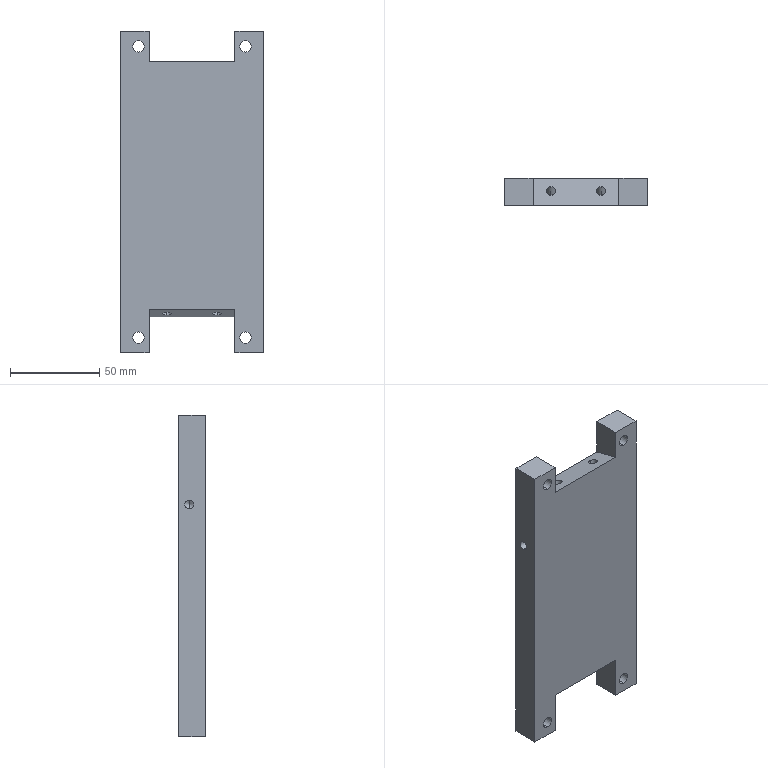Part | SolidWorks | features BaseBody 1 | 1 solid | 46 faces | box 80 x 15 x 180 mm | volume 182488 mm3 | cylinder 20 | plane 14 | cone 12 | commonest cylinder face diameters 5 x12 6.4 x8
STEP:
#1=CARTESIAN_POINT('',(14.,12.806,-50.107));
#2=VERTEX_POINT('',#1);
#3=CARTESIAN_POINT('',(14.,10.002,-50.911));
#4=VERTEX_POINT('',#3);
#5=CARTESIAN_POINT('',(14.,10.002,-50.911));
#6=DIRECTION('',(0.,-0.9613,-0.2756));
#7=VECTOR('',#6,1000.);
#8=LINE('',#5,#7);
#9=EDGE_CURVE('',#2,#4,#8,.T.);
#10=ORIENTED_EDGE('',*,*,#9,.F.);
#11=CARTESIAN_POINT('',(14.,14.832,-52.205));
#12=VERTEX_POINT('',#11);
#13=CARTESIAN_POINT('',(14.,14.832,-52.205));
#14=DIRECTION('',(0.,0.6947,-0.7193));
#15=VECTOR('',#14,1000.);
#16=LINE('',#13,#15);
#17=EDGE_CURVE('',#2,#12,#16,.T.);
#18=ORIENTED_EDGE('',*,*,#17,.T.);
#19=CARTESIAN_POINT('',(14.,12.417,-51.558));
#20=DIRECTION('',(0.,-0.2588,-0.9659));
#21=DIRECTION('',(0.,0.9659,-0.2588));
#22=AXIS2_PLACEMENT_3D('',#19,#20,#21);
#23=CIRCLE('',#22,2.5);
#24=EDGE_CURVE('',#12,#4,#23,.T.);
#25=ORIENTED_EDGE('',*,*,#24,.T.);
#26=EDGE_LOOP('',(#10,#18,#25));
#27=FACE_OUTER_BOUND('',#26,.T.);
#28=CARTESIAN_POINT('',(14.,12.417,-51.558));
#29=DIRECTION('',(0.,-0.2588,-0.9659));
#30=DIRECTION('',(0.,0.9659,-0.2588));
#31=AXIS2_PLACEMENT_3D('',#28,#29,#30);
#32=CONICAL_SURFACE('',#31,2.5,1.03);
#33=ADVANCED_FACE('',(#27),#32,.F.);
#34=CARTESIAN_POINT('',(-14.,12.806,-50.107));
#35=VERTEX_POINT('',#34);
#36=CARTESIAN_POINT('',(-14.,10.002,-50.911));
#37=VERTEX_POINT('',#36);
#38=CARTESIAN_POINT('',(-14.,10.002,-50.911));
#39=DIRECTION('',(0.,-0.9613,-0.2756));
#40=VECTOR('',#39,1000.);
#41=LINE('',#38,#40);
#42=EDGE_CURVE('',#35,#37,#41,.T.);
#43=ORIENTED_EDGE('',*,*,#42,.F.);
#44=CARTESIAN_POINT('',(-14.,14.832,-52.205));
#45=VERTEX_POINT('',#44);
#46=CARTESIAN_POINT('',(-14.,14.832,-52.205));
#47=DIRECTION('',(0.,0.6947,-0.7193));
#48=VECTOR('',#47,1000.);
#49=LINE('',#46,#48);
#50=EDGE_CURVE('',#35,#45,#49,.T.);
#51=ORIENTED_EDGE('',*,*,#50,.T.);
#52=CARTESIAN_POINT('',(-14.,12.417,-51.558));
#53=DIRECTION('',(0.,-0.2588,-0.9659));
#54=DIRECTION('',(0.,0.9659,-0.2588));
#55=AXIS2_PLACEMENT_3D('',#52,#53,#54);
#56=CIRCLE('',#55,2.5);
#57=EDGE_CURVE('',#45,#37,#56,.T.);
#58=ORIENTED_EDGE('',*,*,#57,.T.);
#59=EDGE_LOOP('',(#43,#51,#58));
#60=FACE_OUTER_BOUND('',#59,.T.);
#61=CARTESIAN_POINT('',(-14.,12.417,-51.558));
#62=DIRECTION('',(0.,-0.2588,-0.9659));
#63=DIRECTION('',(0.,0.9659,-0.2588));
#64=AXIS2_PLACEMENT_3D('',#61,#62,#63);
#65=CONICAL_SURFACE('',#64,2.5,1.03);
#66=ADVANCED_FACE('',(#60),#65,.F.);
#67=CARTESIAN_POINT('',(-21.498,9.,40.));
#68=VERTEX_POINT('',#67);
#69=CARTESIAN_POINT('',(-23.,9.,37.5));
#70=VERTEX_POINT('',#69);
#71=CARTESIAN_POINT('',(-23.,9.,37.5));
#72=DIRECTION('',(-0.515,0.,-0.8572));
#73=VECTOR('',#72,1000.);
#74=LINE('',#71,#73);
#75=EDGE_CURVE('',#68,#70,#74,.T.);
#76=ORIENTED_EDGE('',*,*,#75,.F.);
#77=CARTESIAN_POINT('',(-23.,9.,42.5));
#78=VERTEX_POINT('',#77);
#79=CARTESIAN_POINT('',(-23.,9.,42.5));
#80=DIRECTION('',(-0.515,0.,0.8572));
#81=VECTOR('',#80,1000.);
#82=LINE('',#79,#81);
#83=EDGE_CURVE('',#68,#78,#82,.T.);
#84=ORIENTED_EDGE('',*,*,#83,.T.);
#85=CARTESIAN_POINT('',(-23.,9.,40.));
#86=DIRECTION('',(-1.,0.,0.));
#87=DIRECTION('',(0.,0.,1.));
#88=AXIS2_PLACEMENT_3D('',#85,#86,#87);
#89=CIRCLE('',#88,2.5);
#90=EDGE_CURVE('',#78,#70,#89,.T.);
#91=ORIENTED_EDGE('',*,*,#90,.T.);
#92=EDGE_LOOP('',(#76,#84,#91));
#93=FACE_OUTER_BOUND('',#92,.T.);
#94=CARTESIAN_POINT('',(-23.,9.,40.));
#95=DIRECTION('',(-1.,0.,0.));
#96=DIRECTION('',(0.,0.,1.));
#97=AXIS2_PLACEMENT_3D('',#94,#95,#96);
#98=CONICAL_SURFACE('',#97,2.5,1.03);
#99=ADVANCED_FACE('',(#93),#98,.F.);
#100=CARTESIAN_POINT('',(14.,3.228,53.149));
#101=VERTEX_POINT('',#100);
#102=CARTESIAN_POINT('',(14.,6.032,53.953));
#103=VERTEX_POINT('',#102);
#104=CARTESIAN_POINT('',(14.,6.032,53.953));
#105=DIRECTION('',(0.,0.9613,0.2756));
#106=VECTOR('',#105,1000.);
#107=LINE('',#104,#106);
#108=EDGE_CURVE('',#101,#103,#107,.T.);
#109=ORIENTED_EDGE('',*,*,#108,.F.);
#110=CARTESIAN_POINT('',(14.,1.202,55.247));
#111=VERTEX_POINT('',#110);
#112=CARTESIAN_POINT('',(14.,1.202,55.247));
#113=DIRECTION('',(0.,-0.6947,0.7193));
#114=VECTOR('',#113,1000.);
#115=LINE('',#112,#114);
#116=EDGE_CURVE('',#101,#111,#115,.T.);
#117=ORIENTED_EDGE('',*,*,#116,.T.);
#118=CARTESIAN_POINT('',(14.,3.617,54.6));
#119=DIRECTION('',(0.,0.2588,0.9659));
#120=DIRECTION('',(0.,-0.9659,0.2588));
#121=AXIS2_PLACEMENT_3D('',#118,#119,#120);
#122=CIRCLE('',#121,2.5);
#123=EDGE_CURVE('',#111,#103,#122,.T.);
#124=ORIENTED_EDGE('',*,*,#123,.T.);
#125=EDGE_LOOP('',(#109,#117,#124));
#126=FACE_OUTER_BOUND('',#125,.T.);
#127=CARTESIAN_POINT('',(14.,3.617,54.6));
#128=DIRECTION('',(0.,0.2588,0.9659));
#129=DIRECTION('',(0.,-0.9659,0.2588));
#130=AXIS2_PLACEMENT_3D('',#127,#128,#129);
#131=CONICAL_SURFACE('',#130,2.5,1.03);
#132=ADVANCED_FACE('',(#126),#131,.F.);
#133=CARTESIAN_POINT('',(-14.,3.228,53.149));
#134=VERTEX_POINT('',#133);
#135=CARTESIAN_POINT('',(-14.,6.032,53.953));
#136=VERTEX_POINT('',#135);
#137=CARTESIAN_POINT('',(-14.,6.032,53.953));
#138=DIRECTION('',(0.,0.9613,0.2756));
#139=VECTOR('',#138,1000.);
#140=LINE('',#137,#139);
#141=EDGE_CURVE('',#134,#136,#140,.T.);
#142=ORIENTED_EDGE('',*,*,#141,.F.);
#143=CARTESIAN_POINT('',(-14.,1.202,55.247));
#144=VERTEX_POINT('',#143);
#145=CARTESIAN_POINT('',(-14.,1.202,55.247));
#146=DIRECTION('',(0.,-0.6947,0.7193));
#147=VECTOR('',#146,1000.);
#148=LINE('',#145,#147);
#149=EDGE_CURVE('',#134,#144,#148,.T.);
#150=ORIENTED_EDGE('',*,*,#149,.T.);
#151=CARTESIAN_POINT('',(-14.,3.617,54.6));
#152=DIRECTION('',(0.,0.2588,0.9659));
#153=DIRECTION('',(0.,-0.9659,0.2588));
#154=AXIS2_PLACEMENT_3D('',#151,#152,#153);
#155=CIRCLE('',#154,2.5);
#156=EDGE_CURVE('',#144,#136,#155,.T.);
#157=ORIENTED_EDGE('',*,*,#156,.T.);
#158=EDGE_LOOP('',(#142,#150,#157));
#159=FACE_OUTER_BOUND('',#158,.T.);
#160=CARTESIAN_POINT('',(-14.,3.617,54.6));
#161=DIRECTION('',(0.,0.2588,0.9659));
#162=DIRECTION('',(0.,-0.9659,0.2588));
#163=AXIS2_PLACEMENT_3D('',#160,#161,#162);
#164=CONICAL_SURFACE('',#163,2.5,1.03);
#165=ADVANCED_FACE('',(#159),#164,.F.);
#166=CARTESIAN_POINT('',(21.498,9.,-60.));
#167=VERTEX_POINT('',#166);
#168=CARTESIAN_POINT('',(23.,9.,-57.5));
#169=VERTEX_POINT('',#168);
#170=CARTESIAN_POINT('',(23.,9.,-57.5));
#171=DIRECTION('',(0.515,0.,0.8572));
#172=VECTOR('',#171,1000.);
#173=LINE('',#170,#172);
#174=EDGE_CURVE('',#167,#169,#173,.T.);
#175=ORIENTED_EDGE('',*,*,#174,.F.);
#176=CARTESIAN_POINT('',(23.,9.,-62.5));
#177=VERTEX_POINT('',#176);
#178=CARTESIAN_POINT('',(23.,9.,-62.5));
#179=DIRECTION('',(0.515,0.,-0.8572));
#180=VECTOR('',#179,1000.);
#181=LINE('',#178,#180);
#182=EDGE_CURVE('',#167,#177,#181,.T.);
#183=ORIENTED_EDGE('',*,*,#182,.T.);
#184=CARTESIAN_POINT('',(23.,9.,-60.));
#185=DIRECTION('',(1.,0.,0.));
#186=DIRECTION('',(0.,0.,-1.));
#187=AXIS2_PLACEMENT_3D('',#184,#185,#186);
#188=CIRCLE('',#187,2.5);
#189=EDGE_CURVE('',#177,#169,#188,.T.);
#190=ORIENTED_EDGE('',*,*,#189,.T.);
#191=EDGE_LOOP('',(#175,#183,#190));
#192=FACE_OUTER_BOUND('',#191,.T.);
#193=CARTESIAN_POINT('',(23.,9.,-60.));
#194=DIRECTION('',(1.,0.,0.));
#195=DIRECTION('',(0.,0.,-1.));
#196=AXIS2_PLACEMENT_3D('',#193,#194,#195);
#197=CONICAL_SURFACE('',#196,2.5,1.03);
#198=ADVANCED_FACE('',(#192),#197,.F.);
#199=CARTESIAN_POINT('',(14.,5.602,-67.332));
#200=VERTEX_POINT('',#199);
#201=CARTESIAN_POINT('',(14.,5.602,-67.332));
#202=DIRECTION('',(0.,-0.2588,-0.9659));
#203=VECTOR('',#202,1000.);
#204=LINE('',#201,#203);
#205=EDGE_CURVE('',#4,#200,#204,.T.);
#206=ORIENTED_EDGE('',*,*,#205,.F.);
#207=ORIENTED_EDGE('',*,*,#24,.F.);
#208=CARTESIAN_POINT('',(14.,10.432,-68.626));
#209=VERTEX_POINT('',#208);
#210=CARTESIAN_POINT('',(14.,10.432,-68.626));
#211=DIRECTION('',(0.,-0.2588,-0.9659));
#212=VECTOR('',#211,1000.);
#213=LINE('',#210,#212);
#214=EDGE_CURVE('',#12,#209,#213,.T.);
#215=ORIENTED_EDGE('',*,*,#214,.T.);
#216=CARTESIAN_POINT('',(14.,8.017,-67.979));
#217=DIRECTION('',(0.,0.2588,0.9659));
#218=DIRECTION('',(0.,0.9659,-0.2588));
#219=AXIS2_PLACEMENT_3D('',#216,#217,#218);
#220=CIRCLE('',#219,2.5);
#221=EDGE_CURVE('',#200,#209,#220,.T.);
#222=ORIENTED_EDGE('',*,*,#221,.F.);
#223=EDGE_LOOP('',(#206,#207,#215,#222));
#224=FACE_OUTER_BOUND('',#223,.T.);
#225=CARTESIAN_POINT('',(14.,8.017,-67.979));
#226=DIRECTION('',(0.,-0.2588,-0.9659));
#227=DIRECTION('',(0.,0.9659,-0.2588));
#228=AXIS2_PLACEMENT_3D('',#225,#226,#227);
#229=CYLINDRICAL_SURFACE('',#228,2.5);
#230=ADVANCED_FACE('',(#224),#229,.F.);
#231=CARTESIAN_POINT('',(-14.,5.602,-67.332));
#232=VERTEX_POINT('',#231);
#233=CARTESIAN_POINT('',(-14.,5.602,-67.332));
#234=DIRECTION('',(0.,-0.2588,-0.9659));
#235=VECTOR('',#234,1000.);
#236=LINE('',#233,#235);
#237=EDGE_CURVE('',#37,#232,#236,.T.);
#238=ORIENTED_EDGE('',*,*,#237,.F.);
#239=ORIENTED_EDGE('',*,*,#57,.F.);
#240=CARTESIAN_POINT('',(-14.,10.432,-68.626));
#241=VERTEX_POINT('',#240);
#242=CARTESIAN_POINT('',(-14.,10.432,-68.626));
#243=DIRECTION('',(0.,-0.2588,-0.9659));
#244=VECTOR('',#243,1000.);
#245=LINE('',#242,#244);
#246=EDGE_CURVE('',#45,#241,#245,.T.);
#247=ORIENTED_EDGE('',*,*,#246,.T.);
#248=CARTESIAN_POINT('',(-14.,8.017,-67.979));
#249=DIRECTION('',(0.,0.2588,0.9659));
#250=DIRECTION('',(0.,0.9659,-0.2588));
#251=AXIS2_PLACEMENT_3D('',#248,#249,#250);
#252=CIRCLE('',#251,2.5);
#253=EDGE_CURVE('',#232,#241,#252,.T.);
#254=ORIENTED_EDGE('',*,*,#253,.F.);
#255=EDGE_LOOP('',(#238,#239,#247,#254));
#256=FACE_OUTER_BOUND('',#255,.T.);
#257=CARTESIAN_POINT('',(-14.,8.017,-67.979));
#258=DIRECTION('',(0.,-0.2588,-0.9659));
#259=DIRECTION('',(0.,0.9659,-0.2588));
#260=AXIS2_PLACEMENT_3D('',#257,#258,#259);
#261=CYLINDRICAL_SURFACE('',#260,2.5);
#262=ADVANCED_FACE('',(#256),#261,.F.);
#263=CARTESIAN_POINT('',(-40.,9.,37.5));
#264=VERTEX_POINT('',#263);
#265=CARTESIAN_POINT('',(-40.,9.,37.5));
#266=DIRECTION('',(-1.,0.,0.));
#267=VECTOR('',#266,1000.);
#268=LINE('',#265,#267);
#269=EDGE_CURVE('',#70,#264,#268,.T.);
#270=ORIENTED_EDGE('',*,*,#269,.F.);
#271=ORIENTED_EDGE('',*,*,#90,.F.);
#272=CARTESIAN_POINT('',(-40.,9.,42.5));
#273=VERTEX_POINT('',#272);
#274=CARTESIAN_POINT('',(-40.,9.,42.5));
#275=DIRECTION('',(-1.,0.,0.));
#276=VECTOR('',#275,1000.);
#277=LINE('',#274,#276);
#278=EDGE_CURVE('',#78,#273,#277,.T.);
#279=ORIENTED_EDGE('',*,*,#278,.T.);
#280=CARTESIAN_POINT('',(-40.,9.,40.));
#281=DIRECTION('',(-1.,0.,0.));
#282=DIRECTION('',(0.,0.,1.));
#283=AXIS2_PLACEMENT_3D('',#280,#281,#282);
#284=CIRCLE('',#283,2.5);
#285=EDGE_CURVE('',#273,#264,#284,.T.);
#286=ORIENTED_EDGE('',*,*,#285,.T.);
#287=EDGE_LOOP('',(#270,#271,#279,#286));
#288=FACE_OUTER_BOUND('',#287,.T.);
#289=CARTESIAN_POINT('',(-40.,9.,40.));
#290=DIRECTION('',(-1.,0.,0.));
#291=DIRECTION('',(0.,0.,1.));
#292=AXIS2_PLACEMENT_3D('',#289,#290,#291);
#293=CYLINDRICAL_SURFACE('',#292,2.5);
#294=ADVANCED_FACE('',(#288),#293,.F.);
#295=CARTESIAN_POINT('',(14.,10.432,70.374));
#296=VERTEX_POINT('',#295);
#297=CARTESIAN_POINT('',(14.,10.432,70.374));
#298=DIRECTION('',(0.,0.2588,0.9659));
#299=VECTOR('',#298,1000.);
#300=LINE('',#297,#299);
#301=EDGE_CURVE('',#103,#296,#300,.T.);
#302=ORIENTED_EDGE('',*,*,#301,.F.);
#303=ORIENTED_EDGE('',*,*,#123,.F.);
#304=CARTESIAN_POINT('',(14.,5.602,71.668));
#305=VERTEX_POINT('',#304);
#306=CARTESIAN_POINT('',(14.,5.602,71.668));
#307=DIRECTION('',(0.,0.2588,0.9659));
#308=VECTOR('',#307,1000.);
#309=LINE('',#306,#308);
#310=EDGE_CURVE('',#111,#305,#309,.T.);
#311=ORIENTED_EDGE('',*,*,#310,.T.);
#312=CARTESIAN_POINT('',(14.,8.017,71.021));
#313=DIRECTION('',(0.,-0.2588,-0.9659));
#314=DIRECTION('',(0.,-0.9659,0.2588));
#315=AXIS2_PLACEMENT_3D('',#312,#313,#314);
#316=CIRCLE('',#315,2.5);
#317=EDGE_CURVE('',#296,#305,#316,.T.);
#318=ORIENTED_EDGE('',*,*,#317,.F.);
#319=EDGE_LOOP('',(#302,#303,#311,#318));
#320=FACE_OUTER_BOUND('',#319,.T.);
#321=CARTESIAN_POINT('',(14.,8.017,71.021));
#322=DIRECTION('',(0.,0.2588,0.9659));
#323=DIRECTION('',(0.,-0.9659,0.2588));
#324=AXIS2_PLACEMENT_3D('',#321,#322,#323);
#325=CYLINDRICAL_SURFACE('',#324,2.5);
#326=ADVANCED_FACE('',(#320),#325,.F.);
#327=CARTESIAN_POINT('',(-14.,10.432,70.374));
#328=VERTEX_POINT('',#327);
#329=CARTESIAN_POINT('',(-14.,10.432,70.374));
#330=DIRECTION('',(0.,0.2588,0.9659));
#331=VECTOR('',#330,1000.);
#332=LINE('',#329,#331);
#333=EDGE_CURVE('',#136,#328,#332,.T.);
#334=ORIENTED_EDGE('',*,*,#333,.F.);
#335=ORIENTED_EDGE('',*,*,#156,.F.);
#336=CARTESIAN_POINT('',(-14.,5.602,71.668));
#337=VERTEX_POINT('',#336);
#338=CARTESIAN_POINT('',(-14.,5.602,71.668));
#339=DIRECTION('',(0.,0.2588,0.9659));
#340=VECTOR('',#339,1000.);
#341=LINE('',#338,#340);
#342=EDGE_CURVE('',#144,#337,#341,.T.);
#343=ORIENTED_EDGE('',*,*,#342,.T.);
#344=CARTESIAN_POINT('',(-14.,8.017,71.021));
#345=DIRECTION('',(0.,-0.2588,-0.9659));
#346=DIRECTION('',(0.,-0.9659,0.2588));
#347=AXIS2_PLACEMENT_3D('',#344,#345,#346);
#348=CIRCLE('',#347,2.5);
#349=EDGE_CURVE('',#328,#337,#348,.T.);
#350=ORIENTED_EDGE('',*,*,#349,.F.);
#351=EDGE_LOOP('',(#334,#335,#343,#350));
#352=FACE_OUTER_BOUND('',#351,.T.);
#353=CARTESIAN_POINT('',(-14.,8.017,71.021));
#354=DIRECTION('',(0.,0.2588,0.9659));
#355=DIRECTION('',(0.,-0.9659,0.2588));
#356=AXIS2_PLACEMENT_3D('',#353,#354,#355);
#357=CYLINDRICAL_SURFACE('',#356,2.5);
#358=ADVANCED_FACE('',(#352),#357,.F.);
#359=CARTESIAN_POINT('',(40.,9.,-57.5));
#360=VERTEX_POINT('',#359);
#361=CARTESIAN_POINT('',(40.,9.,-57.5));
#362=DIRECTION('',(1.,0.,0.));
#363=VECTOR('',#362,1000.);
#364=LINE('',#361,#363);
#365=EDGE_CURVE('',#169,#360,#364,.T.);
#366=ORIENTED_EDGE('',*,*,#365,.F.);
#367=ORIENTED_EDGE('',*,*,#189,.F.);
#368=CARTESIAN_POINT('',(40.,9.,-62.5));
#369=VERTEX_POINT('',#368);
#370=CARTESIAN_POINT('',(40.,9.,-62.5));
#371=DIRECTION('',(1.,0.,0.));
#372=VECTOR('',#371,1000.);
#373=LINE('',#370,#372);
#374=EDGE_CURVE('',#177,#369,#373,.T.);
#375=ORIENTED_EDGE('',*,*,#374,.T.);
#376=CARTESIAN_POINT('',(40.,9.,-60.));
#377=DIRECTION('',(1.,0.,0.));
#378=DIRECTION('',(0.,0.,-1.));
#379=AXIS2_PLACEMENT_3D('',#376,#377,#378);
#380=CIRCLE('',#379,2.5);
#381=EDGE_CURVE('',#369,#360,#380,.T.);
#382=ORIENTED_EDGE('',*,*,#381,.T.);
#383=EDGE_LOOP('',(#366,#367,#375,#382));
#384=FACE_OUTER_BOUND('',#383,.T.);
#385=CARTESIAN_POINT('',(40.,9.,-60.));
#386=DIRECTION('',(1.,0.,0.));
#387=DIRECTION('',(0.,0.,-1.));
#388=AXIS2_PLACEMENT_3D('',#385,#386,#387);
#389=CYLINDRICAL_SURFACE('',#388,2.5);
#390=ADVANCED_FACE('',(#384),#389,.F.);
#391=CARTESIAN_POINT('',(-30.,15.,-78.3));
#392=VERTEX_POINT('',#391);
#393=CARTESIAN_POINT('',(-30.,15.,-84.7));
#394=VERTEX_POINT('',#393);
#395=CARTESIAN_POINT('',(-30.,15.,-81.5));
#396=DIRECTION('',(0.,-1.,0.));
#397=DIRECTION('',(0.,0.,1.));
#398=AXIS2_PLACEMENT_3D('',#395,#396,#397);
#399=CIRCLE('',#398,3.2);
#400=EDGE_CURVE('',#392,#394,#399,.T.);
#401=ORIENTED_EDGE('',*,*,#400,.T.);
#402=CARTESIAN_POINT('',(-30.,15.,-81.5));
#403=DIRECTION('',(0.,-1.,0.));
#404=DIRECTION('',(0.,0.,1.));
#405=AXIS2_PLACEMENT_3D('',#402,#403,#404);
#406=CIRCLE('',#405,3.2);
#407=EDGE_CURVE('',#394,#392,#406,.T.);
#408=ORIENTED_EDGE('',*,*,#407,.T.);
#409=EDGE_LOOP('',(#401,#408));
#410=FACE_BOUND('',#409,.T.);
#411=CARTESIAN_POINT('',(30.,15.,-78.3));
#412=VERTEX_POINT('',#411);
#413=CARTESIAN_POINT('',(30.,15.,-84.7));
#414=VERTEX_POINT('',#413);
#415=CARTESIAN_POINT('',(30.,15.,-81.5));
#416=DIRECTION('',(0.,-1.,0.));
#417=DIRECTION('',(0.,0.,1.));
#418=AXIS2_PLACEMENT_3D('',#415,#416,#417);
#419=CIRCLE('',#418,3.2);
#420=EDGE_CURVE('',#412,#414,#419,.T.);
#421=ORIENTED_EDGE('',*,*,#420,.T.);
#422=CARTESIAN_POINT('',(30.,15.,-81.5));
#423=DIRECTION('',(0.,-1.,0.));
#424=DIRECTION('',(0.,0.,1.));
#425=AXIS2_PLACEMENT_3D('',#422,#423,#424);
#426=CIRCLE('',#425,3.2);
#427=EDGE_CURVE('',#414,#412,#426,.T.);
#428=ORIENTED_EDGE('',*,*,#427,.T.);
#429=EDGE_LOOP('',(#421,#428));
#430=FACE_BOUND('',#429,.T.);
#431=CARTESIAN_POINT('',(-30.,15.,84.7));
#432=VERTEX_POINT('',#431);
#433=CARTESIAN_POINT('',(-30.,15.,78.3));
#434=VERTEX_POINT('',#433);
#435=CARTESIAN_POINT('',(-30.,15.,81.5));
#436=DIRECTION('',(0.,-1.,0.));
#437=DIRECTION('',(0.,0.,1.));
#438=AXIS2_PLACEMENT_3D('',#435,#436,#437);
#439=CIRCLE('',#438,3.2);
#440=EDGE_CURVE('',#432,#434,#439,.T.);
#441=ORIENTED_EDGE('',*,*,#440,.T.);
#442=CARTESIAN_POINT('',(-30.,15.,81.5));
#443=DIRECTION('',(0.,-1.,0.));
#444=DIRECTION('',(0.,0.,1.));
#445=AXIS2_PLACEMENT_3D('',#442,#443,#444);
#446=CIRCLE('',#445,3.2);
#447=EDGE_CURVE('',#434,#432,#446,.T.);
#448=ORIENTED_EDGE('',*,*,#447,.T.);
#449=EDGE_LOOP('',(#441,#448));
#450=FACE_BOUND('',#449,.T.);
#451=CARTESIAN_POINT('',(30.,15.,84.7));
#452=VERTEX_POINT('',#451);
#453=CARTESIAN_POINT('',(30.,15.,78.3));
#454=VERTEX_POINT('',#453);
#455=CARTESIAN_POINT('',(30.,15.,81.5));
#456=DIRECTION('',(0.,-1.,0.));
#457=DIRECTION('',(0.,0.,1.));
#458=AXIS2_PLACEMENT_3D('',#455,#456,#457);
#459=CIRCLE('',#458,3.2);
#460=EDGE_CURVE('',#452,#454,#459,.T.);
#461=ORIENTED_EDGE('',*,*,#460,.T.);
#462=CARTESIAN_POINT('',(30.,15.,81.5));
#463=DIRECTION('',(0.,-1.,0.));
#464=DIRECTION('',(0.,0.,1.));
#465=AXIS2_PLACEMENT_3D('',#462,#463,#464);
#466=CIRCLE('',#465,3.2);
#467=EDGE_CURVE('',#454,#452,#466,.T.);
#468=ORIENTED_EDGE('',*,*,#467,.T.);
#469=EDGE_LOOP('',(#461,#468));
#470=FACE_BOUND('',#469,.T.);
#471=CARTESIAN_POINT('',(24.,15.,90.));
#472=VERTEX_POINT('',#471);
#473=CARTESIAN_POINT('',(24.,15.,69.15));
#474=VERTEX_POINT('',#473);
#475=CARTESIAN_POINT('',(24.,15.,0.));
#476=DIRECTION('',(0.,0.,-1.));
#477=VECTOR('',#476,1000.);
#478=LINE('',#475,#477);
#479=EDGE_CURVE('',#472,#474,#478,.T.);
#480=ORIENTED_EDGE('',*,*,#479,.F.);
#481=CARTESIAN_POINT('',(40.,15.,90.));
#482=VERTEX_POINT('',#481);
#483=CARTESIAN_POINT('',(-40.,15.,90.));
#484=DIRECTION('',(1.,0.,0.));
#485=VECTOR('',#484,1000.);
#486=LINE('',#483,#485);
#487=EDGE_CURVE('',#472,#482,#486,.T.);
#488=ORIENTED_EDGE('',*,*,#487,.T.);
#489=CARTESIAN_POINT('',(40.,15.,-90.));
#490=VERTEX_POINT('',#489);
#491=CARTESIAN_POINT('',(40.,15.,-90.));
#492=DIRECTION('',(0.,0.,-1.));
#493=VECTOR('',#492,1000.);
#494=LINE('',#491,#493);
#495=EDGE_CURVE('',#482,#490,#494,.T.);
#496=ORIENTED_EDGE('',*,*,#495,.T.);
#497=CARTESIAN_POINT('',(24.,15.,-90.));
#498=VERTEX_POINT('',#497);
#499=CARTESIAN_POINT('',(-40.,15.,-90.));
#500=DIRECTION('',(-1.,0.,0.));
#501=VECTOR('',#500,1000.);
#502=LINE('',#499,#501);
#503=EDGE_CURVE('',#490,#498,#502,.T.);
#504=ORIENTED_EDGE('',*,*,#503,.T.);
#505=CARTESIAN_POINT('',(24.,15.,-69.85));
#506=VERTEX_POINT('',#505);
#507=CARTESIAN_POINT('',(24.,15.,0.));
#508=DIRECTION('',(0.,0.,1.));
#509=VECTOR('',#508,1000.);
#510=LINE('',#507,#509);
#511=EDGE_CURVE('',#498,#506,#510,.T.);
#512=ORIENTED_EDGE('',*,*,#511,.T.);
#513=CARTESIAN_POINT('',(-24.,15.,-69.85));
#514=VERTEX_POINT('',#513);
#515=CARTESIAN_POINT('',(24.,15.,-69.85));
#516=DIRECTION('',(1.,0.,0.));
#517=VECTOR('',#516,1000.);
#518=LINE('',#515,#517);
#519=EDGE_CURVE('',#514,#506,#518,.T.);
#520=ORIENTED_EDGE('',*,*,#519,.F.);
#521=CARTESIAN_POINT('',(-24.,15.,-90.));
#522=VERTEX_POINT('',#521);
#523=CARTESIAN_POINT('',(-24.,15.,0.));
#524=DIRECTION('',(0.,0.,1.));
#525=VECTOR('',#524,1000.);
#526=LINE('',#523,#525);
#527=EDGE_CURVE('',#522,#514,#526,.T.);
#528=ORIENTED_EDGE('',*,*,#527,.F.);
#529=CARTESIAN_POINT('',(-40.,15.,-90.));
#530=VERTEX_POINT('',#529);
#531=CARTESIAN_POINT('',(-40.,15.,-90.));
#532=DIRECTION('',(-1.,0.,0.));
#533=VECTOR('',#532,1000.);
#534=LINE('',#531,#533);
#535=EDGE_CURVE('',#522,#530,#534,.T.);
#536=ORIENTED_EDGE('',*,*,#535,.T.);
#537=CARTESIAN_POINT('',(-40.,15.,90.));
#538=VERTEX_POINT('',#537);
#539=CARTESIAN_POINT('',(-40.,15.,-90.));
#540=DIRECTION('',(0.,0.,1.));
#541=VECTOR('',#540,1000.);
#542=LINE('',#539,#541);
#543=EDGE_CURVE('',#530,#538,#542,.T.);
#544=ORIENTED_EDGE('',*,*,#543,.T.);
#545=CARTESIAN_POINT('',(-24.,15.,90.));
#546=VERTEX_POINT('',#545);
#547=CARTESIAN_POINT('',(-40.,15.,90.));
#548=DIRECTION('',(1.,0.,0.));
#549=VECTOR('',#548,1000.);
#550=LINE('',#547,#549);
#551=EDGE_CURVE('',#538,#546,#550,.T.);
#552=ORIENTED_EDGE('',*,*,#551,.T.);
#553=CARTESIAN_POINT('',(-24.,15.,69.15));
#554=VERTEX_POINT('',#553);
#555=CARTESIAN_POINT('',(-24.,15.,0.));
#556=DIRECTION('',(0.,0.,-1.));
#557=VECTOR('',#556,1000.);
#558=LINE('',#555,#557);
#559=EDGE_CURVE('',#546,#554,#558,.T.);
#560=ORIENTED_EDGE('',*,*,#559,.T.);
#561=CARTESIAN_POINT('',(24.,15.,69.15));
#562=DIRECTION('',(-1.,0.,0.));
#563=VECTOR('',#562,1000.);
#564=LINE('',#561,#563);
#565=EDGE_CURVE('',#474,#554,#564,.T.);
#566=ORIENTED_EDGE('',*,*,#565,.F.);
#567=EDGE_LOOP('',(#480,#488,#496,#504,#512,#520,#528,#536,#544,#552,#560,#566));
#568=FACE_OUTER_BOUND('',#567,.T.);
#569=CARTESIAN_POINT('',(0.,15.,0.));
#570=DIRECTION('',(0.,1.,0.));
#571=DIRECTION('',(1.,0.,0.));
#572=AXIS2_PLACEMENT_3D('',#569,#570,#571);
#573=PLANE('',#572);
#574=ADVANCED_FACE('',(#410,#430,#450,#470,#568),#573,.T.);
#575=CARTESIAN_POINT('',(14.,8.017,-67.979));
#576=DIRECTION('',(0.,0.2588,0.9659));
#577=DIRECTION('',(0.,0.9659,-0.2588));
#578=AXIS2_PLACEMENT_3D('',#575,#576,#577);
#579=CIRCLE('',#578,2.5);
#580=EDGE_CURVE('',#209,#200,#579,.T.);
#581=ORIENTED_EDGE('',*,*,#580,.T.);
#582=ORIENTED_EDGE('',*,*,#221,.T.);
#583=EDGE_LOOP('',(#581,#582));
#584=FACE_BOUND('',#583,.T.);
#585=CARTESIAN_POINT('',(-14.,8.017,-67.979));
#586=DIRECTION('',(0.,0.2588,0.9659));
#587=DIRECTION('',(0.,0.9659,-0.2588));
#588=AXIS2_PLACEMENT_3D('',#585,#586,#587);
#589=CIRCLE('',#588,2.5);
#590=EDGE_CURVE('',#241,#232,#589,.T.);
#591=ORIENTED_EDGE('',*,*,#590,.T.);
#592=ORIENTED_EDGE('',*,*,#253,.T.);
#593=EDGE_LOOP('',(#591,#592));
#594=FACE_BOUND('',#593,.T.);
#595=ORIENTED_EDGE('',*,*,#519,.T.);
#596=CARTESIAN_POINT('',(24.,0.,-65.831));
#597=VERTEX_POINT('',#596);
#598=CARTESIAN_POINT('',(24.,15.,-69.85));
#599=DIRECTION('',(0.,-0.9659,0.2588));
#600=VECTOR('',#599,1000.);
#601=LINE('',#598,#600);
#602=EDGE_CURVE('',#506,#597,#601,.T.);
#603=ORIENTED_EDGE('',*,*,#602,.T.);
#604=CARTESIAN_POINT('',(-24.,0.,-65.831));
#605=VERTEX_POINT('',#604);
#606=CARTESIAN_POINT('',(0.,0.,-65.831));
#607=DIRECTION('',(-1.,0.,0.));
#608=VECTOR('',#607,1000.);
#609=LINE('',#606,#608);
#610=EDGE_CURVE('',#597,#605,#609,.T.);
#611=ORIENTED_EDGE('',*,*,#610,.T.);
#612=CARTESIAN_POINT('',(-24.,15.,-69.85));
#613=DIRECTION('',(0.,-0.9659,0.2588));
#614=VECTOR('',#613,1000.);
#615=LINE('',#612,#614);
#616=EDGE_CURVE('',#514,#605,#615,.T.);
#617=ORIENTED_EDGE('',*,*,#616,.F.);
#618=EDGE_LOOP('',(#595,#603,#611,#617));
#619=FACE_OUTER_BOUND('',#618,.T.);
#620=CARTESIAN_POINT('',(24.,0.,-65.831));
#621=DIRECTION('',(0.,-0.2588,-0.9659));
#622=DIRECTION('',(0.,-0.9659,0.2588));
#623=AXIS2_PLACEMENT_3D('',#620,#621,#622);
#624=PLANE('',#623);
#625=ADVANCED_FACE('',(#584,#594,#619),#624,.T.);
#626=CARTESIAN_POINT('',(-24.,0.,-90.));
#627=VERTEX_POINT('',#626);
#628=CARTESIAN_POINT('',(-24.,0.,0.));
#629=DIRECTION('',(0.,0.,-1.));
#630=VECTOR('',#629,1000.);
#631=LINE('',#628,#630);
#632=EDGE_CURVE('',#605,#627,#631,.T.);
#633=ORIENTED_EDGE('',*,*,#632,.T.);
#634=CARTESIAN_POINT('',(-24.,15.,-90.));
#635=DIRECTION('',(0.,1.,0.));
#636=VECTOR('',#635,1000.);
#637=LINE('',#634,#636);
#638=EDGE_CURVE('',#627,#522,#637,.T.);
#639=ORIENTED_EDGE('',*,*,#638,.T.);
#640=ORIENTED_EDGE('',*,*,#527,.T.);
#641=ORIENTED_EDGE('',*,*,#616,.T.);
#642=EDGE_LOOP('',(#633,#639,#640,#641));
#643=FACE_OUTER_BOUND('',#642,.T.);
#644=CARTESIAN_POINT('',(-24.,0.,0.));
#645=DIRECTION('',(1.,0.,0.));
#646=DIRECTION('',(0.,1.,0.));
#647=AXIS2_PLACEMENT_3D('',#644,#645,#646);
#648=PLANE('',#647);
#649=ADVANCED_FACE('',(#643),#648,.T.);
#650=CARTESIAN_POINT('',(-40.,0.,-90.));
#651=VERTEX_POINT('',#650);
#652=CARTESIAN_POINT('',(-40.,15.,-90.));
#653=DIRECTION('',(0.,1.,0.));
#654=VECTOR('',#653,1000.);
#655=LINE('',#652,#654);
#656=EDGE_CURVE('',#651,#530,#655,.T.);
#657=ORIENTED_EDGE('',*,*,#656,.T.);
#658=ORIENTED_EDGE('',*,*,#535,.F.);
#659=ORIENTED_EDGE('',*,*,#638,.F.);
#660=CARTESIAN_POINT('',(0.,0.,-90.));
#661=DIRECTION('',(-1.,0.,0.));
#662=VECTOR('',#661,1000.);
#663=LINE('',#660,#662);
#664=EDGE_CURVE('',#627,#651,#663,.T.);
#665=ORIENTED_EDGE('',*,*,#664,.T.);
#666=EDGE_LOOP('',(#657,#658,#659,#665));
#667=FACE_OUTER_BOUND('',#666,.T.);
#668=CARTESIAN_POINT('',(-40.,15.,-90.));
#669=DIRECTION('',(0.,0.,1.));
#670=DIRECTION('',(1.,0.,0.));
#671=AXIS2_PLACEMENT_3D('',#668,#669,#670);
#672=PLANE('',#671);
#673=ADVANCED_FACE('',(#667),#672,.F.);
#674=ORIENTED_EDGE('',*,*,#285,.F.);
#675=CARTESIAN_POINT('',(-40.,9.,40.));
#676=DIRECTION('',(-1.,0.,0.));
#677=DIRECTION('',(0.,0.,1.));
#678=AXIS2_PLACEMENT_3D('',#675,#676,#677);
#679=CIRCLE('',#678,2.5);
#680=EDGE_CURVE('',#264,#273,#679,.T.);
#681=ORIENTED_EDGE('',*,*,#680,.F.);
#682=EDGE_LOOP('',(#674,#681));
#683=FACE_BOUND('',#682,.T.);
#684=ORIENTED_EDGE('',*,*,#543,.F.);
#685=ORIENTED_EDGE('',*,*,#656,.F.);
#686=CARTESIAN_POINT('',(-40.,0.,90.));
#687=VERTEX_POINT('',#686);
#688=CARTESIAN_POINT('',(-40.,0.,0.));
#689=DIRECTION('',(0.,0.,1.));
#690=VECTOR('',#689,1000.);
#691=LINE('',#688,#690);
#692=EDGE_CURVE('',#651,#687,#691,.T.);
#693=ORIENTED_EDGE('',*,*,#692,.T.);
#694=CARTESIAN_POINT('',(-40.,15.,90.));
#695=DIRECTION('',(0.,1.,0.));
#696=VECTOR('',#695,1000.);
#697=LINE('',#694,#696);
#698=EDGE_CURVE('',#687,#538,#697,.T.);
#699=ORIENTED_EDGE('',*,*,#698,.T.);
#700=EDGE_LOOP('',(#684,#685,#693,#699));
#701=FACE_OUTER_BOUND('',#700,.T.);
#702=CARTESIAN_POINT('',(-40.,15.,-90.));
#703=DIRECTION('',(1.,0.,0.));
#704=DIRECTION('',(0.,0.,-1.));
#705=AXIS2_PLACEMENT_3D('',#702,#703,#704);
#706=PLANE('',#705);
#707=ADVANCED_FACE('',(#683,#701),#706,.F.);
#708=ORIENTED_EDGE('',*,*,#551,.F.);
#709=ORIENTED_EDGE('',*,*,#698,.F.);
#710=CARTESIAN_POINT('',(-24.,0.,90.));
#711=VERTEX_POINT('',#710);
#712=CARTESIAN_POINT('',(0.,0.,90.));
#713=DIRECTION('',(1.,0.,0.));
#714=VECTOR('',#713,1000.);
#715=LINE('',#712,#714);
#716=EDGE_CURVE('',#687,#711,#715,.T.);
#717=ORIENTED_EDGE('',*,*,#716,.T.);
#718=CARTESIAN_POINT('',(-24.,0.,90.));
#719=DIRECTION('',(0.,1.,0.));
#720=VECTOR('',#719,1000.);
#721=LINE('',#718,#720);
#722=EDGE_CURVE('',#711,#546,#721,.T.);
#723=ORIENTED_EDGE('',*,*,#722,.T.);
#724=EDGE_LOOP('',(#708,#709,#717,#723));
#725=FACE_OUTER_BOUND('',#724,.T.);
#726=CARTESIAN_POINT('',(-40.,15.,90.));
#727=DIRECTION('',(0.,0.,-1.));
#728=DIRECTION('',(0.,-1.,0.));
#729=AXIS2_PLACEMENT_3D('',#726,#727,#728);
#730=PLANE('',#729);
#731=ADVANCED_FACE('',(#725),#730,.F.);
#732=ORIENTED_EDGE('',*,*,#559,.F.);
#733=ORIENTED_EDGE('',*,*,#722,.F.);
#734=CARTESIAN_POINT('',(-24.,0.,73.169));
#735=VERTEX_POINT('',#734);
#736=CARTESIAN_POINT('',(-24.,0.,0.));
#737=DIRECTION('',(0.,0.,-1.));
#738=VECTOR('',#737,1000.);
#739=LINE('',#736,#738);
#740=EDGE_CURVE('',#711,#735,#739,.T.);
#741=ORIENTED_EDGE('',*,*,#740,.T.);
#742=CARTESIAN_POINT('',(-24.,0.,73.169));
#743=DIRECTION('',(0.,-0.9659,0.2588));
#744=VECTOR('',#743,1000.);
#745=LINE('',#742,#744);
#746=EDGE_CURVE('',#554,#735,#745,.T.);
#747=ORIENTED_EDGE('',*,*,#746,.F.);
#748=EDGE_LOOP('',(#732,#733,#741,#747));
#749=FACE_OUTER_BOUND('',#748,.T.);
#750=CARTESIAN_POINT('',(-24.,0.,0.));
#751=DIRECTION('',(-1.,0.,0.));
#752=DIRECTION('',(0.,0.,1.));
#753=AXIS2_PLACEMENT_3D('',#750,#751,#752);
#754=PLANE('',#753);
#755=ADVANCED_FACE('',(#749),#754,.F.);
#756=CARTESIAN_POINT('',(14.,8.017,71.021));
#757=DIRECTION('',(0.,-0.2588,-0.9659));
#758=DIRECTION('',(0.,-0.9659,0.2588));
#759=AXIS2_PLACEMENT_3D('',#756,#757,#758);
#760=CIRCLE('',#759,2.5);
#761=EDGE_CURVE('',#305,#296,#760,.T.);
#762=ORIENTED_EDGE('',*,*,#761,.T.);
#763=ORIENTED_EDGE('',*,*,#317,.T.);
#764=EDGE_LOOP('',(#762,#763));
#765=FACE_BOUND('',#764,.T.);
#766=CARTESIAN_POINT('',(-14.,8.017,71.021));
#767=DIRECTION('',(0.,-0.2588,-0.9659));
#768=DIRECTION('',(0.,-0.9659,0.2588));
#769=AXIS2_PLACEMENT_3D('',#766,#767,#768);
#770=CIRCLE('',#769,2.5);
#771=EDGE_CURVE('',#337,#328,#770,.T.);
#772=ORIENTED_EDGE('',*,*,#771,.T.);
#773=ORIENTED_EDGE('',*,*,#349,.T.);
#774=EDGE_LOOP('',(#772,#773));
#775=FACE_BOUND('',#774,.T.);
#776=CARTESIAN_POINT('',(24.,0.,73.169));
#777=VERTEX_POINT('',#776);
#778=CARTESIAN_POINT('',(0.,0.,73.169));
#779=DIRECTION('',(1.,0.,0.));
#780=VECTOR('',#779,1000.);
#781=LINE('',#778,#780);
#782=EDGE_CURVE('',#735,#777,#781,.T.);
#783=ORIENTED_EDGE('',*,*,#782,.T.);
#784=CARTESIAN_POINT('',(24.,15.,69.15));
#785=DIRECTION('',(0.,-0.9659,0.2588));
#786=VECTOR('',#785,1000.);
#787=LINE('',#784,#786);
#788=EDGE_CURVE('',#474,#777,#787,.T.);
#789=ORIENTED_EDGE('',*,*,#788,.F.);
#790=ORIENTED_EDGE('',*,*,#565,.T.);
#791=ORIENTED_EDGE('',*,*,#746,.T.);
#792=EDGE_LOOP('',(#783,#789,#790,#791));
#793=FACE_OUTER_BOUND('',#792,.T.);
#794=CARTESIAN_POINT('',(24.,0.,73.169));
#795=DIRECTION('',(0.,0.2588,0.9659));
#796=DIRECTION('',(1.,0.,0.));
#797=AXIS2_PLACEMENT_3D('',#794,#795,#796);
#798=PLANE('',#797);
#799=ADVANCED_FACE('',(#765,#775,#793),#798,.T.);
#800=CARTESIAN_POINT('',(24.,0.,90.));
#801=VERTEX_POINT('',#800);
#802=CARTESIAN_POINT('',(24.,0.,0.));
#803=DIRECTION('',(0.,0.,1.));
#804=VECTOR('',#803,1000.);
#805=LINE('',#802,#804);
#806=EDGE_CURVE('',#777,#801,#805,.T.);
#807=ORIENTED_EDGE('',*,*,#806,.T.);
#808=CARTESIAN_POINT('',(24.,15.,90.));
#809=DIRECTION('',(0.,1.,0.));
#810=VECTOR('',#809,1000.);
#811=LINE('',#808,#810);
#812=EDGE_CURVE('',#801,#472,#811,.T.);
#813=ORIENTED_EDGE('',*,*,#812,.T.);
#814=ORIENTED_EDGE('',*,*,#479,.T.);
#815=ORIENTED_EDGE('',*,*,#788,.T.);
#816=EDGE_LOOP('',(#807,#813,#814,#815));
#817=FACE_OUTER_BOUND('',#816,.T.);
#818=CARTESIAN_POINT('',(24.,0.,0.));
#819=DIRECTION('',(-1.,0.,0.));
#820=DIRECTION('',(0.,0.,1.));
#821=AXIS2_PLACEMENT_3D('',#818,#819,#820);
#822=PLANE('',#821);
#823=ADVANCED_FACE('',(#817),#822,.T.);
#824=CARTESIAN_POINT('',(40.,0.,90.));
#825=VERTEX_POINT('',#824);
#826=CARTESIAN_POINT('',(40.,15.,90.));
#827=DIRECTION('',(0.,1.,0.));
#828=VECTOR('',#827,1000.);
#829=LINE('',#826,#828);
#830=EDGE_CURVE('',#825,#482,#829,.T.);
#831=ORIENTED_EDGE('',*,*,#830,.T.);
#832=ORIENTED_EDGE('',*,*,#487,.F.);
#833=ORIENTED_EDGE('',*,*,#812,.F.);
#834=CARTESIAN_POINT('',(0.,0.,90.));
#835=DIRECTION('',(1.,0.,0.));
#836=VECTOR('',#835,1000.);
#837=LINE('',#834,#836);
#838=EDGE_CURVE('',#801,#825,#837,.T.);
#839=ORIENTED_EDGE('',*,*,#838,.T.);
#840=EDGE_LOOP('',(#831,#832,#833,#839));
#841=FACE_OUTER_BOUND('',#840,.T.);
#842=CARTESIAN_POINT('',(-40.,15.,90.));
#843=DIRECTION('',(0.,0.,-1.));
#844=DIRECTION('',(0.,-1.,0.));
#845=AXIS2_PLACEMENT_3D('',#842,#843,#844);
#846=PLANE('',#845);
#847=ADVANCED_FACE('',(#841),#846,.F.);
#848=ORIENTED_EDGE('',*,*,#381,.F.);
#849=CARTESIAN_POINT('',(40.,9.,-60.));
#850=DIRECTION('',(1.,0.,0.));
#851=DIRECTION('',(0.,0.,-1.));
#852=AXIS2_PLACEMENT_3D('',#849,#850,#851);
#853=CIRCLE('',#852,2.5);
#854=EDGE_CURVE('',#360,#369,#853,.T.);
#855=ORIENTED_EDGE('',*,*,#854,.F.);
#856=EDGE_LOOP('',(#848,#855));
#857=FACE_BOUND('',#856,.T.);
#858=ORIENTED_EDGE('',*,*,#495,.F.);
#859=ORIENTED_EDGE('',*,*,#830,.F.);
#860=CARTESIAN_POINT('',(40.,0.,-90.));
#861=VERTEX_POINT('',#860);
#862=CARTESIAN_POINT('',(40.,0.,0.));
#863=DIRECTION('',(0.,0.,-1.));
#864=VECTOR('',#863,1000.);
#865=LINE('',#862,#864);
#866=EDGE_CURVE('',#825,#861,#865,.T.);
#867=ORIENTED_EDGE('',*,*,#866,.T.);
#868=CARTESIAN_POINT('',(40.,15.,-90.));
#869=DIRECTION('',(0.,1.,0.));
#870=VECTOR('',#869,1000.);
#871=LINE('',#868,#870);
#872=EDGE_CURVE('',#861,#490,#871,.T.);
#873=ORIENTED_EDGE('',*,*,#872,.T.);
#874=EDGE_LOOP('',(#858,#859,#867,#873));
#875=FACE_OUTER_BOUND('',#874,.T.);
#876=CARTESIAN_POINT('',(40.,15.,-90.));
#877=DIRECTION('',(-1.,0.,0.));
#878=DIRECTION('',(0.,1.,0.));
#879=AXIS2_PLACEMENT_3D('',#876,#877,#878);
#880=PLANE('',#879);
#881=ADVANCED_FACE('',(#857,#875),#880,.F.);
#882=ORIENTED_EDGE('',*,*,#503,.F.);
#883=ORIENTED_EDGE('',*,*,#872,.F.);
#884=CARTESIAN_POINT('',(24.,0.,-90.));
#885=VERTEX_POINT('',#884);
#886=CARTESIAN_POINT('',(0.,0.,-90.));
#887=DIRECTION('',(-1.,0.,0.));
#888=VECTOR('',#887,1000.);
#889=LINE('',#886,#888);
#890=EDGE_CURVE('',#861,#885,#889,.T.);
#891=ORIENTED_EDGE('',*,*,#890,.T.);
#892=CARTESIAN_POINT('',(24.,0.,-90.));
#893=DIRECTION('',(0.,1.,0.));
#894=VECTOR('',#893,1000.);
#895=LINE('',#892,#894);
#896=EDGE_CURVE('',#885,#498,#895,.T.);
#897=ORIENTED_EDGE('',*,*,#896,.T.);
#898=EDGE_LOOP('',(#882,#883,#891,#897));
#899=FACE_OUTER_BOUND('',#898,.T.);
#900=CARTESIAN_POINT('',(-40.,15.,-90.));
#901=DIRECTION('',(0.,0.,1.));
#902=DIRECTION('',(1.,0.,0.));
#903=AXIS2_PLACEMENT_3D('',#900,#901,#902);
#904=PLANE('',#903);
#905=ADVANCED_FACE('',(#899),#904,.F.);
#906=ORIENTED_EDGE('',*,*,#511,.F.);
#907=ORIENTED_EDGE('',*,*,#896,.F.);
#908=CARTESIAN_POINT('',(24.,0.,0.));
#909=DIRECTION('',(0.,0.,1.));
#910=VECTOR('',#909,1000.);
#911=LINE('',#908,#910);
#912=EDGE_CURVE('',#885,#597,#911,.T.);
#913=ORIENTED_EDGE('',*,*,#912,.T.);
#914=ORIENTED_EDGE('',*,*,#602,.F.);
#915=EDGE_LOOP('',(#906,#907,#913,#914));
#916=FACE_OUTER_BOUND('',#915,.T.);
#917=CARTESIAN_POINT('',(24.,0.,0.));
#918=DIRECTION('',(1.,0.,0.));
#919=DIRECTION('',(0.,1.,0.));
#920=AXIS2_PLACEMENT_3D('',#917,#918,#919);
#921=PLANE('',#920);
#922=ADVANCED_FACE('',(#916),#921,.F.);
#923=CARTESIAN_POINT('',(-30.,0.,-84.7));
#924=VERTEX_POINT('',#923);
#925=CARTESIAN_POINT('',(-30.,15.,-84.7));
#926=DIRECTION('',(0.,1.,0.));
#927=VECTOR('',#926,1000.);
#928=LINE('',#925,#927);
#929=EDGE_CURVE('',#924,#394,#928,.T.);
#930=ORIENTED_EDGE('',*,*,#929,.F.);
#931=CARTESIAN_POINT('',(-30.,0.,-78.3));
#932=VERTEX_POINT('',#931);
#933=CARTESIAN_POINT('',(-30.,0.,-81.5));
#934=DIRECTION('',(0.,-1.,0.));
#935=DIRECTION('',(0.,0.,1.));
#936=AXIS2_PLACEMENT_3D('',#933,#934,#935);
#937=CIRCLE('',#936,3.2);
#938=EDGE_CURVE('',#924,#932,#937,.T.);
#939=ORIENTED_EDGE('',*,*,#938,.T.);
#940=CARTESIAN_POINT('',(-30.,15.,-78.3));
#941=DIRECTION('',(0.,1.,0.));
#942=VECTOR('',#941,1000.);
#943=LINE('',#940,#942);
#944=EDGE_CURVE('',#932,#392,#943,.T.);
#945=ORIENTED_EDGE('',*,*,#944,.T.);
#946=ORIENTED_EDGE('',*,*,#407,.F.);
#947=EDGE_LOOP('',(#930,#939,#945,#946));
#948=FACE_OUTER_BOUND('',#947,.T.);
#949=CARTESIAN_POINT('',(-30.,15.,-81.5));
#950=DIRECTION('',(0.,1.,0.));
#951=DIRECTION('',(0.,0.,1.));
#952=AXIS2_PLACEMENT_3D('',#949,#950,#951);
#953=CYLINDRICAL_SURFACE('',#952,3.2);
#954=ADVANCED_FACE('',(#948),#953,.F.);
#955=CARTESIAN_POINT('',(30.,0.,-84.7));
#956=VERTEX_POINT('',#955);
#957=CARTESIAN_POINT('',(30.,15.,-84.7));
#958=DIRECTION('',(0.,1.,0.));
#959=VECTOR('',#958,1000.);
#960=LINE('',#957,#959);
#961=EDGE_CURVE('',#956,#414,#960,.T.);
#962=ORIENTED_EDGE('',*,*,#961,.F.);
#963=CARTESIAN_POINT('',(30.,0.,-78.3));
#964=VERTEX_POINT('',#963);
#965=CARTESIAN_POINT('',(30.,0.,-81.5));
#966=DIRECTION('',(0.,-1.,0.));
#967=DIRECTION('',(0.,0.,1.));
#968=AXIS2_PLACEMENT_3D('',#965,#966,#967);
#969=CIRCLE('',#968,3.2);
#970=EDGE_CURVE('',#956,#964,#969,.T.);
#971=ORIENTED_EDGE('',*,*,#970,.T.);
#972=CARTESIAN_POINT('',(30.,15.,-78.3));
#973=DIRECTION('',(0.,1.,0.));
#974=VECTOR('',#973,1000.);
#975=LINE('',#972,#974);
#976=EDGE_CURVE('',#964,#412,#975,.T.);
#977=ORIENTED_EDGE('',*,*,#976,.T.);
#978=ORIENTED_EDGE('',*,*,#427,.F.);
#979=EDGE_LOOP('',(#962,#971,#977,#978));
#980=FACE_OUTER_BOUND('',#979,.T.);
#981=CARTESIAN_POINT('',(30.,15.,-81.5));
#982=DIRECTION('',(0.,1.,0.));
#983=DIRECTION('',(0.,0.,1.));
#984=AXIS2_PLACEMENT_3D('',#981,#982,#983);
#985=CYLINDRICAL_SURFACE('',#984,3.2);
#986=ADVANCED_FACE('',(#980),#985,.F.);
#987=CARTESIAN_POINT('',(-30.,0.,78.3));
#988=VERTEX_POINT('',#987);
#989=CARTESIAN_POINT('',(-30.,15.,78.3));
#990=DIRECTION('',(0.,1.,0.));
#991=VECTOR('',#990,1000.);
#992=LINE('',#989,#991);
#993=EDGE_CURVE('',#988,#434,#992,.T.);
#994=ORIENTED_EDGE('',*,*,#993,.F.);
#995=CARTESIAN_POINT('',(-30.,0.,84.7));
#996=VERTEX_POINT('',#995);
#997=CARTESIAN_POINT('',(-30.,0.,81.5));
#998=DIRECTION('',(0.,-1.,0.));
#999=DIRECTION('',(0.,0.,1.));
#1000=AXIS2_PLACEMENT_3D('',#997,#998,#999);
#1001=CIRCLE('',#1000,3.2);
#1002=EDGE_CURVE('',#988,#996,#1001,.T.);
#1003=ORIENTED_EDGE('',*,*,#1002,.T.);
#1004=CARTESIAN_POINT('',(-30.,15.,84.7));
#1005=DIRECTION('',(0.,1.,0.));
#1006=VECTOR('',#1005,1000.);
#1007=LINE('',#1004,#1006);
#1008=EDGE_CURVE('',#996,#432,#1007,.T.);
#1009=ORIENTED_EDGE('',*,*,#1008,.T.);
#1010=ORIENTED_EDGE('',*,*,#447,.F.);
#1011=EDGE_LOOP('',(#994,#1003,#1009,#1010));
#1012=FACE_OUTER_BOUND('',#1011,.T.);
#1013=CARTESIAN_POINT('',(-30.,15.,81.5));
#1014=DIRECTION('',(0.,1.,0.));
#1015=DIRECTION('',(0.,0.,1.));
#1016=AXIS2_PLACEMENT_3D('',#1013,#1014,#1015);
#1017=CYLINDRICAL_SURFACE('',#1016,3.2);
#1018=ADVANCED_FACE('',(#1012),#1017,.F.);
#1019=CARTESIAN_POINT('',(30.,0.,78.3));
#1020=VERTEX_POINT('',#1019);
#1021=CARTESIAN_POINT('',(30.,15.,78.3));
#1022=DIRECTION('',(0.,1.,0.));
#1023=VECTOR('',#1022,1000.);
#1024=LINE('',#1021,#1023);
#1025=EDGE_CURVE('',#1020,#454,#1024,.T.);
#1026=ORIENTED_EDGE('',*,*,#1025,.F.);
#1027=CARTESIAN_POINT('',(30.,0.,84.7));
#1028=VERTEX_POINT('',#1027);
#1029=CARTESIAN_POINT('',(30.,0.,81.5));
#1030=DIRECTION('',(0.,-1.,0.));
#1031=DIRECTION('',(0.,0.,1.));
#1032=AXIS2_PLACEMENT_3D('',#1029,#1030,#1031);
#1033=CIRCLE('',#1032,3.2);
#1034=EDGE_CURVE('',#1020,#1028,#1033,.T.);
#1035=ORIENTED_EDGE('',*,*,#1034,.T.);
#1036=CARTESIAN_POINT('',(30.,15.,84.7));
#1037=DIRECTION('',(0.,1.,0.));
#1038=VECTOR('',#1037,1000.);
#1039=LINE('',#1036,#1038);
#1040=EDGE_CURVE('',#1028,#452,#1039,.T.);
#1041=ORIENTED_EDGE('',*,*,#1040,.T.);
#1042=ORIENTED_EDGE('',*,*,#467,.F.);
#1043=EDGE_LOOP('',(#1026,#1035,#1041,#1042));
#1044=FACE_OUTER_BOUND('',#1043,.T.);
#1045=CARTESIAN_POINT('',(30.,15.,81.5));
#1046=DIRECTION('',(0.,1.,0.));
#1047=DIRECTION('',(0.,0.,1.));
#1048=AXIS2_PLACEMENT_3D('',#1045,#1046,#1047);
#1049=CYLINDRICAL_SURFACE('',#1048,3.2);
#1050=ADVANCED_FACE('',(#1044),#1049,.F.);
#1051=CARTESIAN_POINT('',(-30.,0.,-81.5));
#1052=DIRECTION('',(0.,-1.,0.));
#1053=DIRECTION('',(0.,0.,1.));
#1054=AXIS2_PLACEMENT_3D('',#1051,#1052,#1053);
#1055=CIRCLE('',#1054,3.2);
#1056=EDGE_CURVE('',#932,#924,#1055,.T.);
#1057=ORIENTED_EDGE('',*,*,#1056,.F.);
#1058=ORIENTED_EDGE('',*,*,#938,.F.);
#1059=EDGE_LOOP('',(#1057,#1058));
#1060=FACE_BOUND('',#1059,.T.);
#1061=CARTESIAN_POINT('',(30.,0.,-81.5));
#1062=DIRECTION('',(0.,-1.,0.));
#1063=DIRECTION('',(0.,0.,1.));
#1064=AXIS2_PLACEMENT_3D('',#1061,#1062,#1063);
#1065=CIRCLE('',#1064,3.2);
#1066=EDGE_CURVE('',#964,#956,#1065,.T.);
#1067=ORIENTED_EDGE('',*,*,#1066,.F.);
#1068=ORIENTED_EDGE('',*,*,#970,.F.);
#1069=EDGE_LOOP('',(#1067,#1068));
#1070=FACE_BOUND('',#1069,.T.);
#1071=CARTESIAN_POINT('',(-30.,0.,81.5));
#1072=DIRECTION('',(0.,-1.,0.));
#1073=DIRECTION('',(0.,0.,1.));
#1074=AXIS2_PLACEMENT_3D('',#1071,#1072,#1073);
#1075=CIRCLE('',#1074,3.2);
#1076=EDGE_CURVE('',#996,#988,#1075,.T.);
#1077=ORIENTED_EDGE('',*,*,#1076,.F.);
#1078=ORIENTED_EDGE('',*,*,#1002,.F.);
#1079=EDGE_LOOP('',(#1077,#1078));
#1080=FACE_BOUND('',#1079,.T.);
#1081=CARTESIAN_POINT('',(30.,0.,81.5));
#1082=DIRECTION('',(0.,-1.,0.));
#1083=DIRECTION('',(0.,0.,1.));
#1084=AXIS2_PLACEMENT_3D('',#1081,#1082,#1083);
#1085=CIRCLE('',#1084,3.2);
#1086=EDGE_CURVE('',#1028,#1020,#1085,.T.);
#1087=ORIENTED_EDGE('',*,*,#1086,.F.);
#1088=ORIENTED_EDGE('',*,*,#1034,.F.);
#1089=EDGE_LOOP('',(#1087,#1088));
#1090=FACE_BOUND('',#1089,.T.);
#1091=ORIENTED_EDGE('',*,*,#890,.F.);
#1092=ORIENTED_EDGE('',*,*,#866,.F.);
#1093=ORIENTED_EDGE('',*,*,#838,.F.);
#1094=ORIENTED_EDGE('',*,*,#806,.F.);
#1095=ORIENTED_EDGE('',*,*,#782,.F.);
#1096=ORIENTED_EDGE('',*,*,#740,.F.);
#1097=ORIENTED_EDGE('',*,*,#716,.F.);
#1098=ORIENTED_EDGE('',*,*,#692,.F.);
#1099=ORIENTED_EDGE('',*,*,#664,.F.);
#1100=ORIENTED_EDGE('',*,*,#632,.F.);
#1101=ORIENTED_EDGE('',*,*,#610,.F.);
#1102=ORIENTED_EDGE('',*,*,#912,.F.);
#1103=EDGE_LOOP('',(#1091,#1092,#1093,#1094,#1095,#1096,#1097,#1098,#1099,#1100,#1101,#1102));
#1104=FACE_OUTER_BOUND('',#1103,.T.);
#1105=CARTESIAN_POINT('',(0.,0.,0.));
#1106=DIRECTION('',(0.,1.,0.));
#1107=DIRECTION('',(1.,0.,0.));
#1108=AXIS2_PLACEMENT_3D('',#1105,#1106,#1107);
#1109=PLANE('',#1108);
#1110=ADVANCED_FACE('',(#1060,#1070,#1080,#1090,#1104),#1109,.F.);
#1111=ORIENTED_EDGE('',*,*,#17,.F.);
#1112=ORIENTED_EDGE('',*,*,#9,.T.);
#1113=CARTESIAN_POINT('',(14.,12.417,-51.558));
#1114=DIRECTION('',(0.,-0.2588,-0.9659));
#1115=DIRECTION('',(0.,0.9659,-0.2588));
#1116=AXIS2_PLACEMENT_3D('',#1113,#1114,#1115);
#1117=CIRCLE('',#1116,2.5);
#1118=EDGE_CURVE('',#4,#12,#1117,.T.);
#1119=ORIENTED_EDGE('',*,*,#1118,.T.);
#1120=EDGE_LOOP('',(#1111,#1112,#1119));
#1121=FACE_OUTER_BOUND('',#1120,.T.);
#1122=CARTESIAN_POINT('',(14.,12.417,-51.558));
#1123=DIRECTION('',(0.,-0.2588,-0.9659));
#1124=DIRECTION('',(0.,0.9659,-0.2588));
#1125=AXIS2_PLACEMENT_3D('',#1122,#1123,#1124);
#1126=CONICAL_SURFACE('',#1125,2.5,1.03);
#1127=ADVANCED_FACE('',(#1121),#1126,.F.);
#1128=ORIENTED_EDGE('',*,*,#50,.F.);
#1129=ORIENTED_EDGE('',*,*,#42,.T.);
#1130=CARTESIAN_POINT('',(-14.,12.417,-51.558));
#1131=DIRECTION('',(0.,-0.2588,-0.9659));
#1132=DIRECTION('',(0.,0.9659,-0.2588));
#1133=AXIS2_PLACEMENT_3D('',#1130,#1131,#1132);
#1134=CIRCLE('',#1133,2.5);
#1135=EDGE_CURVE('',#37,#45,#1134,.T.);
#1136=ORIENTED_EDGE('',*,*,#1135,.T.);
#1137=EDGE_LOOP('',(#1128,#1129,#1136));
#1138=FACE_OUTER_BOUND('',#1137,.T.);
#1139=CARTESIAN_POINT('',(-14.,12.417,-51.558));
#1140=DIRECTION('',(0.,-0.2588,-0.9659));
#1141=DIRECTION('',(0.,0.9659,-0.2588));
#1142=AXIS2_PLACEMENT_3D('',#1139,#1140,#1141);
#1143=CONICAL_SURFACE('',#1142,2.5,1.03);
#1144=ADVANCED_FACE('',(#1138),#1143,.F.);
#1145=ORIENTED_EDGE('',*,*,#83,.F.);
#1146=ORIENTED_EDGE('',*,*,#75,.T.);
#1147=CARTESIAN_POINT('',(-23.,9.,40.));
#1148=DIRECTION('',(-1.,0.,0.));
#1149=DIRECTION('',(0.,0.,1.));
#1150=AXIS2_PLACEMENT_3D('',#1147,#1148,#1149);
#1151=CIRCLE('',#1150,2.5);
#1152=EDGE_CURVE('',#70,#78,#1151,.T.);
#1153=ORIENTED_EDGE('',*,*,#1152,.T.);
#1154=EDGE_LOOP('',(#1145,#1146,#1153));
#1155=FACE_OUTER_BOUND('',#1154,.T.);
#1156=CARTESIAN_POINT('',(-23.,9.,40.));
#1157=DIRECTION('',(-1.,0.,0.));
#1158=DIRECTION('',(0.,0.,1.));
#1159=AXIS2_PLACEMENT_3D('',#1156,#1157,#1158);
#1160=CONICAL_SURFACE('',#1159,2.5,1.03);
#1161=ADVANCED_FACE('',(#1155),#1160,.F.);
#1162=ORIENTED_EDGE('',*,*,#116,.F.);
#1163=ORIENTED_EDGE('',*,*,#108,.T.);
#1164=CARTESIAN_POINT('',(14.,3.617,54.6));
#1165=DIRECTION('',(0.,0.2588,0.9659));
#1166=DIRECTION('',(0.,-0.9659,0.2588));
#1167=AXIS2_PLACEMENT_3D('',#1164,#1165,#1166);
#1168=CIRCLE('',#1167,2.5);
#1169=EDGE_CURVE('',#103,#111,#1168,.T.);
#1170=ORIENTED_EDGE('',*,*,#1169,.T.);
#1171=EDGE_LOOP('',(#1162,#1163,#1170));
#1172=FACE_OUTER_BOUND('',#1171,.T.);
#1173=CARTESIAN_POINT('',(14.,3.617,54.6));
#1174=DIRECTION('',(0.,0.2588,0.9659));
#1175=DIRECTION('',(0.,-0.9659,0.2588));
#1176=AXIS2_PLACEMENT_3D('',#1173,#1174,#1175);
#1177=CONICAL_SURFACE('',#1176,2.5,1.03);
#1178=ADVANCED_FACE('',(#1172),#1177,.F.);
#1179=ORIENTED_EDGE('',*,*,#149,.F.);
#1180=ORIENTED_EDGE('',*,*,#141,.T.);
#1181=CARTESIAN_POINT('',(-14.,3.617,54.6));
#1182=DIRECTION('',(0.,0.2588,0.9659));
#1183=DIRECTION('',(0.,-0.9659,0.2588));
#1184=AXIS2_PLACEMENT_3D('',#1181,#1182,#1183);
#1185=CIRCLE('',#1184,2.5);
#1186=EDGE_CURVE('',#136,#144,#1185,.T.);
#1187=ORIENTED_EDGE('',*,*,#1186,.T.);
#1188=EDGE_LOOP('',(#1179,#1180,#1187));
#1189=FACE_OUTER_BOUND('',#1188,.T.);
#1190=CARTESIAN_POINT('',(-14.,3.617,54.6));
#1191=DIRECTION('',(0.,0.2588,0.9659));
#1192=DIRECTION('',(0.,-0.9659,0.2588));
#1193=AXIS2_PLACEMENT_3D('',#1190,#1191,#1192);
#1194=CONICAL_SURFACE('',#1193,2.5,1.03);
#1195=ADVANCED_FACE('',(#1189),#1194,.F.);
#1196=ORIENTED_EDGE('',*,*,#182,.F.);
#1197=ORIENTED_EDGE('',*,*,#174,.T.);
#1198=CARTESIAN_POINT('',(23.,9.,-60.));
#1199=DIRECTION('',(1.,0.,0.));
#1200=DIRECTION('',(0.,0.,-1.));
#1201=AXIS2_PLACEMENT_3D('',#1198,#1199,#1200);
#1202=CIRCLE('',#1201,2.5);
#1203=EDGE_CURVE('',#169,#177,#1202,.T.);
#1204=ORIENTED_EDGE('',*,*,#1203,.T.);
#1205=EDGE_LOOP('',(#1196,#1197,#1204));
#1206=FACE_OUTER_BOUND('',#1205,.T.);
#1207=CARTESIAN_POINT('',(23.,9.,-60.));
#1208=DIRECTION('',(1.,0.,0.));
#1209=DIRECTION('',(0.,0.,-1.));
#1210=AXIS2_PLACEMENT_3D('',#1207,#1208,#1209);
#1211=CONICAL_SURFACE('',#1210,2.5,1.03);
#1212=ADVANCED_FACE('',(#1206),#1211,.F.);
#1213=ORIENTED_EDGE('',*,*,#1118,.F.);
#1214=ORIENTED_EDGE('',*,*,#205,.T.);
#1215=ORIENTED_EDGE('',*,*,#580,.F.);
#1216=ORIENTED_EDGE('',*,*,#214,.F.);
#1217=EDGE_LOOP('',(#1213,#1214,#1215,#1216));
#1218=FACE_OUTER_BOUND('',#1217,.T.);
#1219=CARTESIAN_POINT('',(14.,8.017,-67.979));
#1220=DIRECTION('',(0.,-0.2588,-0.9659));
#1221=DIRECTION('',(0.,0.9659,-0.2588));
#1222=AXIS2_PLACEMENT_3D('',#1219,#1220,#1221);
#1223=CYLINDRICAL_SURFACE('',#1222,2.5);
#1224=ADVANCED_FACE('',(#1218),#1223,.F.);
#1225=ORIENTED_EDGE('',*,*,#1135,.F.);
#1226=ORIENTED_EDGE('',*,*,#237,.T.);
#1227=ORIENTED_EDGE('',*,*,#590,.F.);
#1228=ORIENTED_EDGE('',*,*,#246,.F.);
#1229=EDGE_LOOP('',(#1225,#1226,#1227,#1228));
#1230=FACE_OUTER_BOUND('',#1229,.T.);
#1231=CARTESIAN_POINT('',(-14.,8.017,-67.979));
#1232=DIRECTION('',(0.,-0.2588,-0.9659));
#1233=DIRECTION('',(0.,0.9659,-0.2588));
#1234=AXIS2_PLACEMENT_3D('',#1231,#1232,#1233);
#1235=CYLINDRICAL_SURFACE('',#1234,2.5);
#1236=ADVANCED_FACE('',(#1230),#1235,.F.);
#1237=ORIENTED_EDGE('',*,*,#1152,.F.);
#1238=ORIENTED_EDGE('',*,*,#269,.T.);
#1239=ORIENTED_EDGE('',*,*,#680,.T.);
#1240=ORIENTED_EDGE('',*,*,#278,.F.);
#1241=EDGE_LOOP('',(#1237,#1238,#1239,#1240));
#1242=FACE_OUTER_BOUND('',#1241,.T.);
#1243=CARTESIAN_POINT('',(-40.,9.,40.));
#1244=DIRECTION('',(-1.,0.,0.));
#1245=DIRECTION('',(0.,0.,1.));
#1246=AXIS2_PLACEMENT_3D('',#1243,#1244,#1245);
#1247=CYLINDRICAL_SURFACE('',#1246,2.5);
#1248=ADVANCED_FACE('',(#1242),#1247,.F.);
#1249=ORIENTED_EDGE('',*,*,#1169,.F.);
#1250=ORIENTED_EDGE('',*,*,#301,.T.);
#1251=ORIENTED_EDGE('',*,*,#761,.F.);
#1252=ORIENTED_EDGE('',*,*,#310,.F.);
#1253=EDGE_LOOP('',(#1249,#1250,#1251,#1252));
#1254=FACE_OUTER_BOUND('',#1253,.T.);
#1255=CARTESIAN_POINT('',(14.,8.017,71.021));
#1256=DIRECTION('',(0.,0.2588,0.9659));
#1257=DIRECTION('',(0.,-0.9659,0.2588));
#1258=AXIS2_PLACEMENT_3D('',#1255,#1256,#1257);
#1259=CYLINDRICAL_SURFACE('',#1258,2.5);
#1260=ADVANCED_FACE('',(#1254),#1259,.F.);
#1261=ORIENTED_EDGE('',*,*,#1186,.F.);
#1262=ORIENTED_EDGE('',*,*,#333,.T.);
#1263=ORIENTED_EDGE('',*,*,#771,.F.);
#1264=ORIENTED_EDGE('',*,*,#342,.F.);
#1265=EDGE_LOOP('',(#1261,#1262,#1263,#1264));
#1266=FACE_OUTER_BOUND('',#1265,.T.);
#1267=CARTESIAN_POINT('',(-14.,8.017,71.021));
#1268=DIRECTION('',(0.,0.2588,0.9659));
#1269=DIRECTION('',(0.,-0.9659,0.2588));
#1270=AXIS2_PLACEMENT_3D('',#1267,#1268,#1269);
#1271=CYLINDRICAL_SURFACE('',#1270,2.5);
#1272=ADVANCED_FACE('',(#1266),#1271,.F.);
#1273=ORIENTED_EDGE('',*,*,#1203,.F.);
#1274=ORIENTED_EDGE('',*,*,#365,.T.);
#1275=ORIENTED_EDGE('',*,*,#854,.T.);
#1276=ORIENTED_EDGE('',*,*,#374,.F.);
#1277=EDGE_LOOP('',(#1273,#1274,#1275,#1276));
#1278=FACE_OUTER_BOUND('',#1277,.T.);
#1279=CARTESIAN_POINT('',(40.,9.,-60.));
#1280=DIRECTION('',(1.,0.,0.));
#1281=DIRECTION('',(0.,0.,-1.));
#1282=AXIS2_PLACEMENT_3D('',#1279,#1280,#1281);
#1283=CYLINDRICAL_SURFACE('',#1282,2.5);
#1284=ADVANCED_FACE('',(#1278),#1283,.F.);
#1285=ORIENTED_EDGE('',*,*,#1056,.T.);
#1286=ORIENTED_EDGE('',*,*,#929,.T.);
#1287=ORIENTED_EDGE('',*,*,#400,.F.);
#1288=ORIENTED_EDGE('',*,*,#944,.F.);
#1289=EDGE_LOOP('',(#1285,#1286,#1287,#1288));
#1290=FACE_OUTER_BOUND('',#1289,.T.);
#1291=CARTESIAN_POINT('',(-30.,15.,-81.5));
#1292=DIRECTION('',(0.,1.,0.));
#1293=DIRECTION('',(0.,0.,1.));
#1294=AXIS2_PLACEMENT_3D('',#1291,#1292,#1293);
#1295=CYLINDRICAL_SURFACE('',#1294,3.2);
#1296=ADVANCED_FACE('',(#1290),#1295,.F.);
#1297=ORIENTED_EDGE('',*,*,#1066,.T.);
#1298=ORIENTED_EDGE('',*,*,#961,.T.);
#1299=ORIENTED_EDGE('',*,*,#420,.F.);
#1300=ORIENTED_EDGE('',*,*,#976,.F.);
#1301=EDGE_LOOP('',(#1297,#1298,#1299,#1300));
#1302=FACE_OUTER_BOUND('',#1301,.T.);
#1303=CARTESIAN_POINT('',(30.,15.,-81.5));
#1304=DIRECTION('',(0.,1.,0.));
#1305=DIRECTION('',(0.,0.,1.));
#1306=AXIS2_PLACEMENT_3D('',#1303,#1304,#1305);
#1307=CYLINDRICAL_SURFACE('',#1306,3.2);
#1308=ADVANCED_FACE('',(#1302),#1307,.F.);
#1309=ORIENTED_EDGE('',*,*,#1076,.T.);
#1310=ORIENTED_EDGE('',*,*,#993,.T.);
#1311=ORIENTED_EDGE('',*,*,#440,.F.);
#1312=ORIENTED_EDGE('',*,*,#1008,.F.);
#1313=EDGE_LOOP('',(#1309,#1310,#1311,#1312));
#1314=FACE_OUTER_BOUND('',#1313,.T.);
#1315=CARTESIAN_POINT('',(-30.,15.,81.5));
#1316=DIRECTION('',(0.,1.,0.));
#1317=DIRECTION('',(0.,0.,1.));
#1318=AXIS2_PLACEMENT_3D('',#1315,#1316,#1317);
#1319=CYLINDRICAL_SURFACE('',#1318,3.2);
#1320=ADVANCED_FACE('',(#1314),#1319,.F.);
#1321=ORIENTED_EDGE('',*,*,#1086,.T.);
#1322=ORIENTED_EDGE('',*,*,#1025,.T.);
#1323=ORIENTED_EDGE('',*,*,#460,.F.);
#1324=ORIENTED_EDGE('',*,*,#1040,.F.);
#1325=EDGE_LOOP('',(#1321,#1322,#1323,#1324));
#1326=FACE_OUTER_BOUND('',#1325,.T.);
#1327=CARTESIAN_POINT('',(30.,15.,81.5));
#1328=DIRECTION('',(0.,1.,0.));
#1329=DIRECTION('',(0.,0.,1.));
#1330=AXIS2_PLACEMENT_3D('',#1327,#1328,#1329);
#1331=CYLINDRICAL_SURFACE('',#1330,3.2);
#1332=ADVANCED_FACE('',(#1326),#1331,.F.);
#1333=CLOSED_SHELL('',(#33,#66,#99,#132,#165,#198,#230,#262,#294,#326,#358,#390,#574,#625,#649,#673,#707,#731,#755,#799,#823,#847,#881,#905,#922,#954,#986,#1018,#1050,#1110,#1127,#1144,#1161,#1178,#1195,#1212,#1224,#1236,#1248,#1260,#1272,#1284,#1296,#1308,#1320,#1332));
#1334=MANIFOLD_SOLID_BREP('',#1333);
#1335=CARTESIAN_POINT('',(0.,0.,0.));
#1336=DIRECTION('',(0.,0.,1.));
#1337=DIRECTION('',(1.,0.,0.));
#1338=AXIS2_PLACEMENT_3D('',#1335,#1336,#1337);
#1339=(LENGTH_UNIT()NAMED_UNIT(*)SI_UNIT(.MILLI.,.METRE.));
#1340=UNCERTAINTY_MEASURE_WITH_UNIT(LENGTH_MEASURE(0.00001),#1339,'','');
#1341=(NAMED_UNIT(*)PLANE_ANGLE_UNIT()SI_UNIT($,.RADIAN.));
#1342=(NAMED_UNIT(*)SI_UNIT($,.STERADIAN.)SOLID_ANGLE_UNIT());
#1343=(GEOMETRIC_REPRESENTATION_CONTEXT(3)GLOBAL_UNCERTAINTY_ASSIGNED_CONTEXT((#1340))GLOBAL_UNIT_ASSIGNED_CONTEXT((#1339,#1341,#1342))REPRESENTATION_CONTEXT('',''));
#1344=ADVANCED_BREP_SHAPE_REPRESENTATION('',(#1334,#1338),#1343);